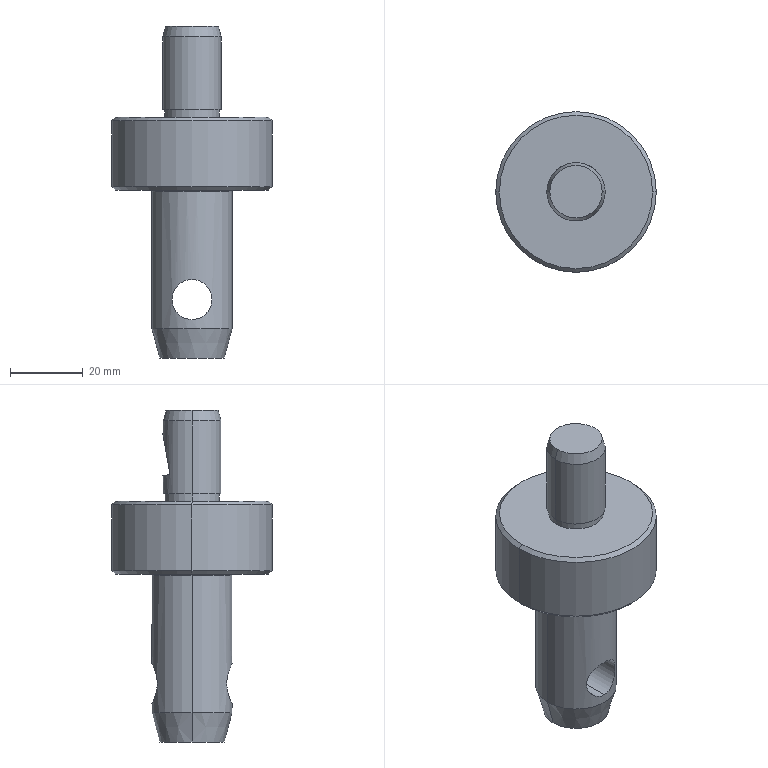Part | STEP file | OP10-107_guide-pin | 1 solid | 27 faces | box 44 x 44 x 91 mm | volume 50039 mm3 | cylinder 10 | cone 8 | plane 7 | torus 2 | commonest cylinder face diameters 11 x2 15 x2 16 x2 22 x2 44 x2